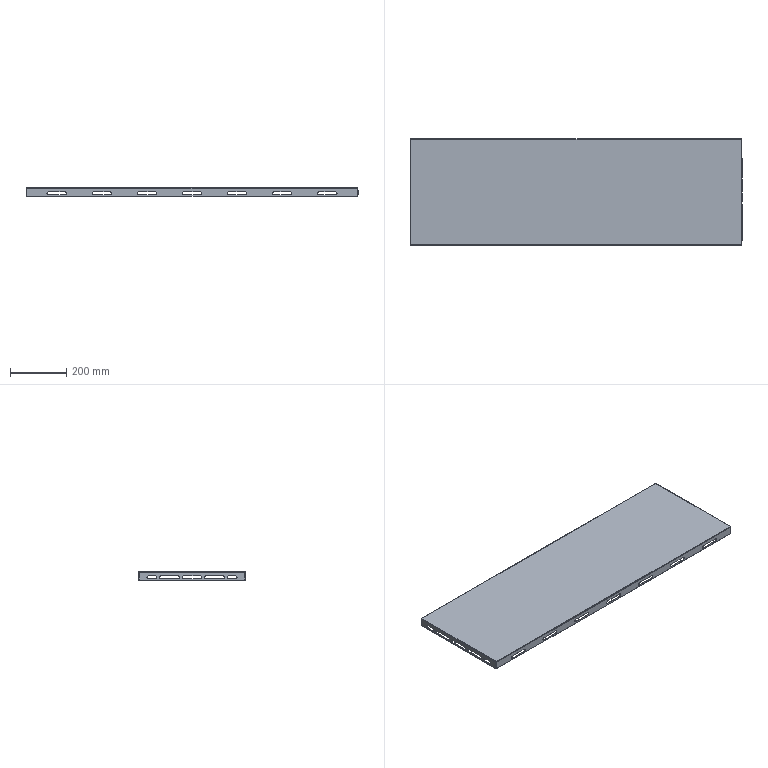Part | SolidWorks | features ICE 2, EdgeFlange 1, FlatPattern 1, SMBaseFlange 1, SheetMetal 1 | 1 solid | 134 faces | box 1179 x 379 x 30 mm | volume 777868 mm3 | plane 70 | cylinder 56 | spline 8 | commonest cylinder face diameters 10 x48 1 x4 4 x4